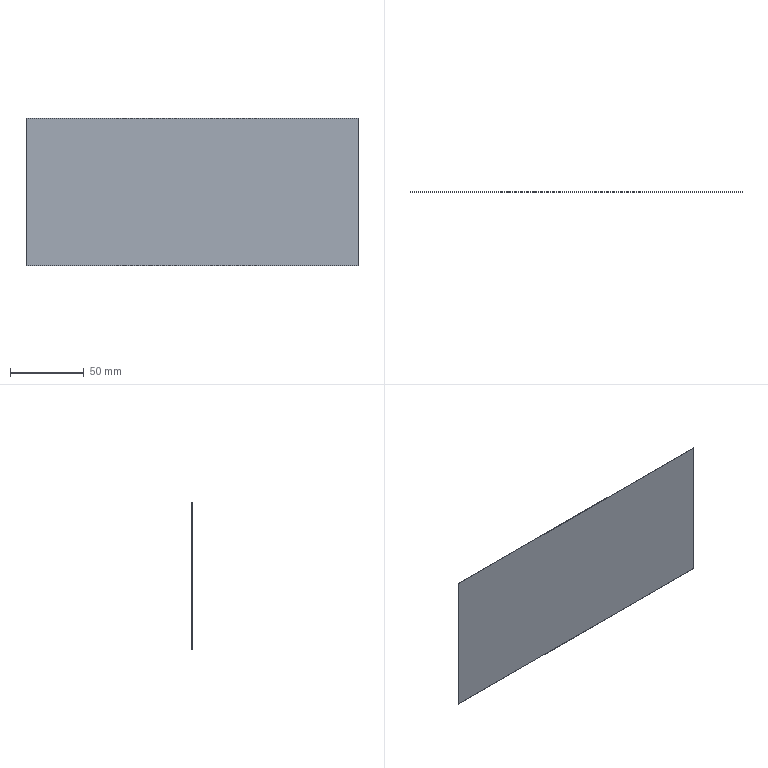Part | STEP file | A14-Product-3 | 1 solid | 6 faces | box 225 x 0.2 x 100 mm | volume 4500 mm3 | plane 6
STEP:
#1=CARTESIAN_POINT('',(0.,0.,0.));
#2=DIRECTION('',(0.,0.,1.));
#3=DIRECTION('',(1.,0.,0.));
#4=AXIS2_PLACEMENT_3D('',#1,#2,#3);
#5=CARTESIAN_POINT('',(112.5,0.,50.));
#6=VERTEX_POINT('',#5);
#7=CARTESIAN_POINT('',(112.5,0.,-50.));
#8=VERTEX_POINT('',#7);
#9=CARTESIAN_POINT('',(112.5,0.,-50.));
#10=DIRECTION('',(0.,0.,-1.));
#11=VECTOR('',#10,1.);
#12=LINE('',#9,#11);
#13=CARTESIAN_POINT('',(112.5,0.2,-50.));
#14=DIRECTION('',(-1.,0.,0.));
#15=DIRECTION('',(0.,0.,1.));
#16=AXIS2_PLACEMENT_3D('',#13,#14,#15);
#17=PLANE('',#16);
#18=CARTESIAN_POINT('',(0.,-0.2));
#19=DIRECTION('',(-1.,0.));
#20=VECTOR('',#19,1.);
#21=LINE('',#18,#20);
#22=(GEOMETRIC_REPRESENTATION_CONTEXT(2)PARAMETRIC_REPRESENTATION_CONTEXT()REPRESENTATION_CONTEXT('',''));
#23=DEFINITIONAL_REPRESENTATION('',(#21),#22);
#24=PCURVE('',#17,#23);
#25=CARTESIAN_POINT('',(0.,0.,0.));
#26=DIRECTION('',(0.,1.,0.));
#27=DIRECTION('',(0.,0.,1.));
#28=AXIS2_PLACEMENT_3D('',#25,#26,#27);
#29=PLANE('',#28);
#30=CARTESIAN_POINT('',(-50.,112.5));
#31=DIRECTION('',(-1.,0.));
#32=VECTOR('',#31,1.);
#33=LINE('',#30,#32);
#34=(GEOMETRIC_REPRESENTATION_CONTEXT(2)PARAMETRIC_REPRESENTATION_CONTEXT()REPRESENTATION_CONTEXT('',''));
#35=DEFINITIONAL_REPRESENTATION('',(#33),#34);
#36=PCURVE('',#29,#35);
#37=SURFACE_CURVE('',#12,(#24,#36),.PCURVE_S1.);
#38=EDGE_CURVE('',#6,#8,#37,.T.);
#39=ORIENTED_EDGE('',*,*,#38,.T.);
#40=CARTESIAN_POINT('',(112.5,0.2,-50.));
#41=VERTEX_POINT('',#40);
#42=CARTESIAN_POINT('',(112.5,0.2,-50.));
#43=DIRECTION('',(0.,-1.,0.));
#44=VECTOR('',#43,1.);
#45=LINE('',#42,#44);
#46=CARTESIAN_POINT('',(0.,0.));
#47=DIRECTION('',(0.,-1.));
#48=VECTOR('',#47,1.);
#49=LINE('',#46,#48);
#50=(GEOMETRIC_REPRESENTATION_CONTEXT(2)PARAMETRIC_REPRESENTATION_CONTEXT()REPRESENTATION_CONTEXT('',''));
#51=DEFINITIONAL_REPRESENTATION('',(#49),#50);
#52=PCURVE('',#17,#51);
#53=CARTESIAN_POINT('',(-112.5,0.2,-50.));
#54=DIRECTION('',(0.,0.,1.));
#55=DIRECTION('',(1.,0.,0.));
#56=AXIS2_PLACEMENT_3D('',#53,#54,#55);
#57=PLANE('',#56);
#58=CARTESIAN_POINT('',(225.,0.));
#59=DIRECTION('',(0.,-1.));
#60=VECTOR('',#59,1.);
#61=LINE('',#58,#60);
#62=(GEOMETRIC_REPRESENTATION_CONTEXT(2)PARAMETRIC_REPRESENTATION_CONTEXT()REPRESENTATION_CONTEXT('',''));
#63=DEFINITIONAL_REPRESENTATION('',(#61),#62);
#64=PCURVE('',#57,#63);
#65=SURFACE_CURVE('',#45,(#52,#64),.PCURVE_S1.);
#66=EDGE_CURVE('',#41,#8,#65,.T.);
#67=ORIENTED_EDGE('',*,*,#66,.F.);
#68=CARTESIAN_POINT('',(112.5,0.2,50.));
#69=VERTEX_POINT('',#68);
#70=CARTESIAN_POINT('',(112.5,0.2,-50.));
#71=DIRECTION('',(0.,0.,-1.));
#72=VECTOR('',#71,1.);
#73=LINE('',#70,#72);
#74=CARTESIAN_POINT('',(0.,0.));
#75=DIRECTION('',(-1.,0.));
#76=VECTOR('',#75,1.);
#77=LINE('',#74,#76);
#78=(GEOMETRIC_REPRESENTATION_CONTEXT(2)PARAMETRIC_REPRESENTATION_CONTEXT()REPRESENTATION_CONTEXT('',''));
#79=DEFINITIONAL_REPRESENTATION('',(#77),#78);
#80=PCURVE('',#17,#79);
#81=CARTESIAN_POINT('',(0.,0.2,0.));
#82=DIRECTION('',(0.,1.,0.));
#83=DIRECTION('',(0.,0.,1.));
#84=AXIS2_PLACEMENT_3D('',#81,#82,#83);
#85=PLANE('',#84);
#86=CARTESIAN_POINT('',(-50.,112.5));
#87=DIRECTION('',(-1.,0.));
#88=VECTOR('',#87,1.);
#89=LINE('',#86,#88);
#90=(GEOMETRIC_REPRESENTATION_CONTEXT(2)PARAMETRIC_REPRESENTATION_CONTEXT()REPRESENTATION_CONTEXT('',''));
#91=DEFINITIONAL_REPRESENTATION('',(#89),#90);
#92=PCURVE('',#85,#91);
#93=SURFACE_CURVE('',#73,(#80,#92),.PCURVE_S1.);
#94=EDGE_CURVE('',#69,#41,#93,.T.);
#95=ORIENTED_EDGE('',*,*,#94,.F.);
#96=CARTESIAN_POINT('',(112.5,0.2,50.));
#97=DIRECTION('',(0.,-1.,0.));
#98=VECTOR('',#97,1.);
#99=LINE('',#96,#98);
#100=CARTESIAN_POINT('',(100.,0.));
#101=DIRECTION('',(0.,-1.));
#102=VECTOR('',#101,1.);
#103=LINE('',#100,#102);
#104=(GEOMETRIC_REPRESENTATION_CONTEXT(2)PARAMETRIC_REPRESENTATION_CONTEXT()REPRESENTATION_CONTEXT('',''));
#105=DEFINITIONAL_REPRESENTATION('',(#103),#104);
#106=PCURVE('',#17,#105);
#107=CARTESIAN_POINT('',(-112.5,0.2,50.));
#108=DIRECTION('',(0.,0.,-1.));
#109=DIRECTION('',(-1.,0.,0.));
#110=AXIS2_PLACEMENT_3D('',#107,#108,#109);
#111=PLANE('',#110);
#112=CARTESIAN_POINT('',(-225.,0.));
#113=DIRECTION('',(0.,-1.));
#114=VECTOR('',#113,1.);
#115=LINE('',#112,#114);
#116=(GEOMETRIC_REPRESENTATION_CONTEXT(2)PARAMETRIC_REPRESENTATION_CONTEXT()REPRESENTATION_CONTEXT('',''));
#117=DEFINITIONAL_REPRESENTATION('',(#115),#116);
#118=PCURVE('',#111,#117);
#119=SURFACE_CURVE('',#99,(#106,#118),.PCURVE_S1.);
#120=EDGE_CURVE('',#69,#6,#119,.T.);
#121=ORIENTED_EDGE('',*,*,#120,.T.);
#122=EDGE_LOOP('',(#39,#67,#95,#121));
#123=FACE_BOUND('',#122,.T.);
#124=ADVANCED_FACE('',(#123),#17,.F.);
#125=CARTESIAN_POINT('',(-112.5,0.,-50.));
#126=VERTEX_POINT('',#125);
#127=CARTESIAN_POINT('',(-112.5,0.,-50.));
#128=DIRECTION('',(-1.,0.,0.));
#129=VECTOR('',#128,1.);
#130=LINE('',#127,#129);
#131=CARTESIAN_POINT('',(0.,-0.2));
#132=DIRECTION('',(-1.,0.));
#133=VECTOR('',#132,1.);
#134=LINE('',#131,#133);
#135=(GEOMETRIC_REPRESENTATION_CONTEXT(2)PARAMETRIC_REPRESENTATION_CONTEXT()REPRESENTATION_CONTEXT('',''));
#136=DEFINITIONAL_REPRESENTATION('',(#134),#135);
#137=PCURVE('',#57,#136);
#138=CARTESIAN_POINT('',(-50.,-112.5));
#139=DIRECTION('',(0.,-1.));
#140=VECTOR('',#139,1.);
#141=LINE('',#138,#140);
#142=(GEOMETRIC_REPRESENTATION_CONTEXT(2)PARAMETRIC_REPRESENTATION_CONTEXT()REPRESENTATION_CONTEXT('',''));
#143=DEFINITIONAL_REPRESENTATION('',(#141),#142);
#144=PCURVE('',#29,#143);
#145=SURFACE_CURVE('',#130,(#137,#144),.PCURVE_S1.);
#146=EDGE_CURVE('',#8,#126,#145,.T.);
#147=ORIENTED_EDGE('',*,*,#146,.T.);
#148=CARTESIAN_POINT('',(-112.5,0.2,-50.));
#149=VERTEX_POINT('',#148);
#150=CARTESIAN_POINT('',(-112.5,0.2,-50.));
#151=DIRECTION('',(0.,-1.,0.));
#152=VECTOR('',#151,1.);
#153=LINE('',#150,#152);
#154=CARTESIAN_POINT('',(0.,0.));
#155=DIRECTION('',(0.,-1.));
#156=VECTOR('',#155,1.);
#157=LINE('',#154,#156);
#158=(GEOMETRIC_REPRESENTATION_CONTEXT(2)PARAMETRIC_REPRESENTATION_CONTEXT()REPRESENTATION_CONTEXT('',''));
#159=DEFINITIONAL_REPRESENTATION('',(#157),#158);
#160=PCURVE('',#57,#159);
#161=CARTESIAN_POINT('',(-112.5,0.2,-50.));
#162=DIRECTION('',(1.,0.,0.));
#163=DIRECTION('',(0.,0.,-1.));
#164=AXIS2_PLACEMENT_3D('',#161,#162,#163);
#165=PLANE('',#164);
#166=CARTESIAN_POINT('',(0.,0.));
#167=DIRECTION('',(0.,-1.));
#168=VECTOR('',#167,1.);
#169=LINE('',#166,#168);
#170=(GEOMETRIC_REPRESENTATION_CONTEXT(2)PARAMETRIC_REPRESENTATION_CONTEXT()REPRESENTATION_CONTEXT('',''));
#171=DEFINITIONAL_REPRESENTATION('',(#169),#170);
#172=PCURVE('',#165,#171);
#173=SURFACE_CURVE('',#153,(#160,#172),.PCURVE_S1.);
#174=EDGE_CURVE('',#149,#126,#173,.T.);
#175=ORIENTED_EDGE('',*,*,#174,.F.);
#176=CARTESIAN_POINT('',(-112.5,0.2,-50.));
#177=DIRECTION('',(-1.,0.,0.));
#178=VECTOR('',#177,1.);
#179=LINE('',#176,#178);
#180=CARTESIAN_POINT('',(0.,0.));
#181=DIRECTION('',(-1.,0.));
#182=VECTOR('',#181,1.);
#183=LINE('',#180,#182);
#184=(GEOMETRIC_REPRESENTATION_CONTEXT(2)PARAMETRIC_REPRESENTATION_CONTEXT()REPRESENTATION_CONTEXT('',''));
#185=DEFINITIONAL_REPRESENTATION('',(#183),#184);
#186=PCURVE('',#57,#185);
#187=CARTESIAN_POINT('',(-50.,-112.5));
#188=DIRECTION('',(0.,-1.));
#189=VECTOR('',#188,1.);
#190=LINE('',#187,#189);
#191=(GEOMETRIC_REPRESENTATION_CONTEXT(2)PARAMETRIC_REPRESENTATION_CONTEXT()REPRESENTATION_CONTEXT('',''));
#192=DEFINITIONAL_REPRESENTATION('',(#190),#191);
#193=PCURVE('',#85,#192);
#194=SURFACE_CURVE('',#179,(#186,#193),.PCURVE_S1.);
#195=EDGE_CURVE('',#41,#149,#194,.T.);
#196=ORIENTED_EDGE('',*,*,#195,.F.);
#197=ORIENTED_EDGE('',*,*,#66,.T.);
#198=EDGE_LOOP('',(#147,#175,#196,#197));
#199=FACE_BOUND('',#198,.T.);
#200=ADVANCED_FACE('',(#199),#57,.F.);
#201=CARTESIAN_POINT('',(-112.5,0.,50.));
#202=VERTEX_POINT('',#201);
#203=CARTESIAN_POINT('',(-112.5,0.,-50.));
#204=DIRECTION('',(0.,0.,1.));
#205=VECTOR('',#204,1.);
#206=LINE('',#203,#205);
#207=CARTESIAN_POINT('',(0.,-0.2));
#208=DIRECTION('',(-1.,0.));
#209=VECTOR('',#208,1.);
#210=LINE('',#207,#209);
#211=(GEOMETRIC_REPRESENTATION_CONTEXT(2)PARAMETRIC_REPRESENTATION_CONTEXT()REPRESENTATION_CONTEXT('',''));
#212=DEFINITIONAL_REPRESENTATION('',(#210),#211);
#213=PCURVE('',#165,#212);
#214=CARTESIAN_POINT('',(-50.,-112.5));
#215=DIRECTION('',(1.,0.));
#216=VECTOR('',#215,1.);
#217=LINE('',#214,#216);
#218=(GEOMETRIC_REPRESENTATION_CONTEXT(2)PARAMETRIC_REPRESENTATION_CONTEXT()REPRESENTATION_CONTEXT('',''));
#219=DEFINITIONAL_REPRESENTATION('',(#217),#218);
#220=PCURVE('',#29,#219);
#221=SURFACE_CURVE('',#206,(#213,#220),.PCURVE_S1.);
#222=EDGE_CURVE('',#126,#202,#221,.T.);
#223=ORIENTED_EDGE('',*,*,#222,.T.);
#224=CARTESIAN_POINT('',(-112.5,0.2,50.));
#225=VERTEX_POINT('',#224);
#226=CARTESIAN_POINT('',(-112.5,0.2,50.));
#227=DIRECTION('',(0.,-1.,0.));
#228=VECTOR('',#227,1.);
#229=LINE('',#226,#228);
#230=CARTESIAN_POINT('',(-100.,0.));
#231=DIRECTION('',(0.,-1.));
#232=VECTOR('',#231,1.);
#233=LINE('',#230,#232);
#234=(GEOMETRIC_REPRESENTATION_CONTEXT(2)PARAMETRIC_REPRESENTATION_CONTEXT()REPRESENTATION_CONTEXT('',''));
#235=DEFINITIONAL_REPRESENTATION('',(#233),#234);
#236=PCURVE('',#165,#235);
#237=CARTESIAN_POINT('',(0.,0.));
#238=DIRECTION('',(0.,-1.));
#239=VECTOR('',#238,1.);
#240=LINE('',#237,#239);
#241=(GEOMETRIC_REPRESENTATION_CONTEXT(2)PARAMETRIC_REPRESENTATION_CONTEXT()REPRESENTATION_CONTEXT('',''));
#242=DEFINITIONAL_REPRESENTATION('',(#240),#241);
#243=PCURVE('',#111,#242);
#244=SURFACE_CURVE('',#229,(#236,#243),.PCURVE_S1.);
#245=EDGE_CURVE('',#225,#202,#244,.T.);
#246=ORIENTED_EDGE('',*,*,#245,.F.);
#247=CARTESIAN_POINT('',(-112.5,0.2,-50.));
#248=DIRECTION('',(0.,0.,1.));
#249=VECTOR('',#248,1.);
#250=LINE('',#247,#249);
#251=CARTESIAN_POINT('',(0.,0.));
#252=DIRECTION('',(-1.,0.));
#253=VECTOR('',#252,1.);
#254=LINE('',#251,#253);
#255=(GEOMETRIC_REPRESENTATION_CONTEXT(2)PARAMETRIC_REPRESENTATION_CONTEXT()REPRESENTATION_CONTEXT('',''));
#256=DEFINITIONAL_REPRESENTATION('',(#254),#255);
#257=PCURVE('',#165,#256);
#258=CARTESIAN_POINT('',(-50.,-112.5));
#259=DIRECTION('',(1.,0.));
#260=VECTOR('',#259,1.);
#261=LINE('',#258,#260);
#262=(GEOMETRIC_REPRESENTATION_CONTEXT(2)PARAMETRIC_REPRESENTATION_CONTEXT()REPRESENTATION_CONTEXT('',''));
#263=DEFINITIONAL_REPRESENTATION('',(#261),#262);
#264=PCURVE('',#85,#263);
#265=SURFACE_CURVE('',#250,(#257,#264),.PCURVE_S1.);
#266=EDGE_CURVE('',#149,#225,#265,.T.);
#267=ORIENTED_EDGE('',*,*,#266,.F.);
#268=ORIENTED_EDGE('',*,*,#174,.T.);
#269=EDGE_LOOP('',(#223,#246,#267,#268));
#270=FACE_BOUND('',#269,.T.);
#271=ADVANCED_FACE('',(#270),#165,.F.);
#272=CARTESIAN_POINT('',(-112.5,0.,50.));
#273=DIRECTION('',(1.,0.,0.));
#274=VECTOR('',#273,1.);
#275=LINE('',#272,#274);
#276=CARTESIAN_POINT('',(0.,-0.2));
#277=DIRECTION('',(-1.,0.));
#278=VECTOR('',#277,1.);
#279=LINE('',#276,#278);
#280=(GEOMETRIC_REPRESENTATION_CONTEXT(2)PARAMETRIC_REPRESENTATION_CONTEXT()REPRESENTATION_CONTEXT('',''));
#281=DEFINITIONAL_REPRESENTATION('',(#279),#280);
#282=PCURVE('',#111,#281);
#283=CARTESIAN_POINT('',(50.,-112.5));
#284=DIRECTION('',(0.,1.));
#285=VECTOR('',#284,1.);
#286=LINE('',#283,#285);
#287=(GEOMETRIC_REPRESENTATION_CONTEXT(2)PARAMETRIC_REPRESENTATION_CONTEXT()REPRESENTATION_CONTEXT('',''));
#288=DEFINITIONAL_REPRESENTATION('',(#286),#287);
#289=PCURVE('',#29,#288);
#290=SURFACE_CURVE('',#275,(#282,#289),.PCURVE_S1.);
#291=EDGE_CURVE('',#202,#6,#290,.T.);
#292=ORIENTED_EDGE('',*,*,#291,.T.);
#293=ORIENTED_EDGE('',*,*,#120,.F.);
#294=CARTESIAN_POINT('',(-112.5,0.2,50.));
#295=DIRECTION('',(1.,0.,0.));
#296=VECTOR('',#295,1.);
#297=LINE('',#294,#296);
#298=CARTESIAN_POINT('',(0.,0.));
#299=DIRECTION('',(-1.,0.));
#300=VECTOR('',#299,1.);
#301=LINE('',#298,#300);
#302=(GEOMETRIC_REPRESENTATION_CONTEXT(2)PARAMETRIC_REPRESENTATION_CONTEXT()REPRESENTATION_CONTEXT('',''));
#303=DEFINITIONAL_REPRESENTATION('',(#301),#302);
#304=PCURVE('',#111,#303);
#305=CARTESIAN_POINT('',(50.,-112.5));
#306=DIRECTION('',(0.,1.));
#307=VECTOR('',#306,1.);
#308=LINE('',#305,#307);
#309=(GEOMETRIC_REPRESENTATION_CONTEXT(2)PARAMETRIC_REPRESENTATION_CONTEXT()REPRESENTATION_CONTEXT('',''));
#310=DEFINITIONAL_REPRESENTATION('',(#308),#309);
#311=PCURVE('',#85,#310);
#312=SURFACE_CURVE('',#297,(#304,#311),.PCURVE_S1.);
#313=EDGE_CURVE('',#225,#69,#312,.T.);
#314=ORIENTED_EDGE('',*,*,#313,.F.);
#315=ORIENTED_EDGE('',*,*,#245,.T.);
#316=EDGE_LOOP('',(#292,#293,#314,#315));
#317=FACE_BOUND('',#316,.T.);
#318=ADVANCED_FACE('',(#317),#111,.F.);
#319=ORIENTED_EDGE('',*,*,#94,.T.);
#320=ORIENTED_EDGE('',*,*,#195,.T.);
#321=ORIENTED_EDGE('',*,*,#266,.T.);
#322=ORIENTED_EDGE('',*,*,#313,.T.);
#323=EDGE_LOOP('',(#319,#320,#321,#322));
#324=FACE_BOUND('',#323,.T.);
#325=ADVANCED_FACE('',(#324),#85,.T.);
#326=ORIENTED_EDGE('',*,*,#38,.F.);
#327=ORIENTED_EDGE('',*,*,#291,.F.);
#328=ORIENTED_EDGE('',*,*,#222,.F.);
#329=ORIENTED_EDGE('',*,*,#146,.F.);
#330=EDGE_LOOP('',(#326,#327,#328,#329));
#331=FACE_BOUND('',#330,.T.);
#332=ADVANCED_FACE('',(#331),#29,.F.);
#333=CLOSED_SHELL('',(#124,#200,#271,#318,#325,#332));
#334=MANIFOLD_SOLID_BREP('',#333);
#335=(LENGTH_UNIT()NAMED_UNIT(*)SI_UNIT(.MILLI.,.METRE.));
#336=UNCERTAINTY_MEASURE_WITH_UNIT(LENGTH_MEASURE(0.0000001),#335,'','');
#337=(NAMED_UNIT(*)PLANE_ANGLE_UNIT()SI_UNIT($,.RADIAN.));
#338=(NAMED_UNIT(*)SI_UNIT($,.STERADIAN.)SOLID_ANGLE_UNIT());
#339=(GEOMETRIC_REPRESENTATION_CONTEXT(3)GLOBAL_UNCERTAINTY_ASSIGNED_CONTEXT((#336))GLOBAL_UNIT_ASSIGNED_CONTEXT((#335,#337,#338))REPRESENTATION_CONTEXT('',''));
#340=ADVANCED_BREP_SHAPE_REPRESENTATION('',(#4,#334),#339);